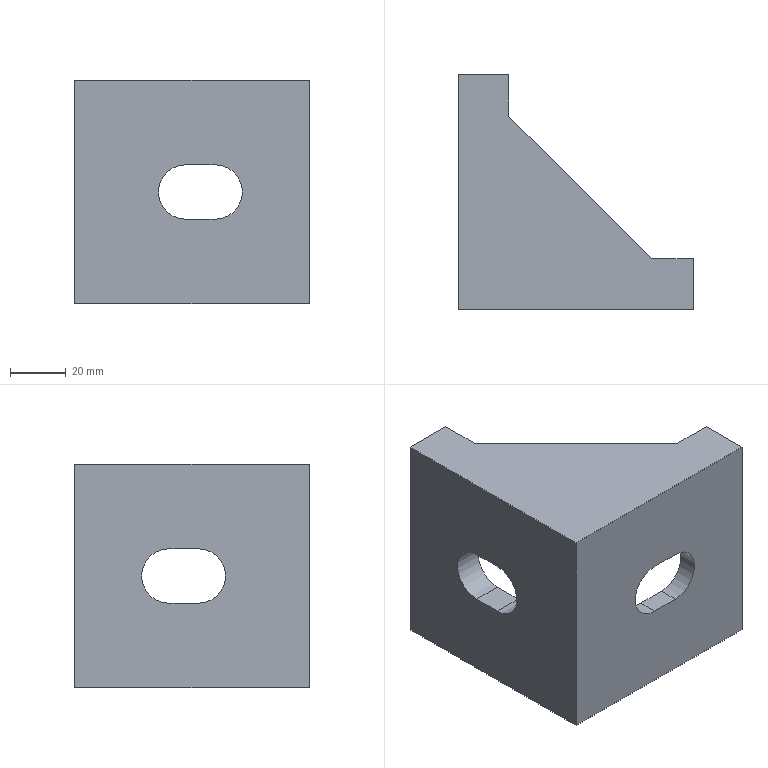Part | STEP file | jiaoma80 | 1 solid | 24 faces | box 84 x 84 x 80 mm | volume 134159 mm3 | plane 20 | cylinder 4 | commonest cylinder face diameters 19.5 x4